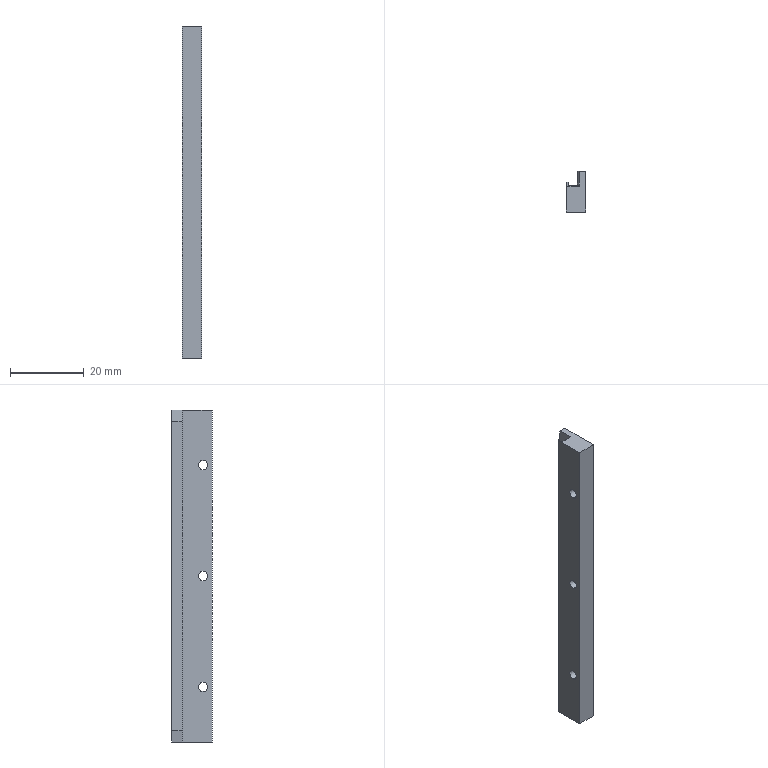Part | NX | features BREP 1 | 1 solid | 22 faces | box 5.3 x 11 x 89.8 mm | volume 4191 mm3 | plane 16 | cylinder 6 | commonest cylinder face diameters 2.5 x6
STEP:
#1=CARTESIAN_POINT('',(3.,11.,41.9));
#2=VERTEX_POINT('',#1);
#3=CARTESIAN_POINT('',(3.5,11.,44.9));
#4=VERTEX_POINT('',#3);
#5=CARTESIAN_POINT('',(3.5,11.,44.9));
#6=DIRECTION('',(0.1644,0.,0.9864));
#7=VECTOR('',#6,1000.);
#8=LINE('',#5,#7);
#9=EDGE_CURVE('',#2,#4,#8,.T.);
#10=ORIENTED_EDGE('',*,*,#9,.F.);
#11=CARTESIAN_POINT('',(3.,7.3,41.9));
#12=VERTEX_POINT('',#11);
#13=CARTESIAN_POINT('',(3.,11.,41.9));
#14=DIRECTION('',(0.,1.,0.));
#15=VECTOR('',#14,1000.);
#16=LINE('',#13,#15);
#17=EDGE_CURVE('',#12,#2,#16,.T.);
#18=ORIENTED_EDGE('',*,*,#17,.F.);
#19=CARTESIAN_POINT('',(3.45,7.3,44.6));
#20=VERTEX_POINT('',#19);
#21=CARTESIAN_POINT('',(3.486,7.3,44.819));
#22=DIRECTION('',(-0.1644,0.,-0.9864));
#23=VECTOR('',#22,1000.);
#24=LINE('',#21,#23);
#25=EDGE_CURVE('',#20,#12,#24,.T.);
#26=ORIENTED_EDGE('',*,*,#25,.F.);
#27=CARTESIAN_POINT('',(3.5,7.,44.9));
#28=VERTEX_POINT('',#27);
#29=CARTESIAN_POINT('',(4.075,3.548,48.352));
#30=DIRECTION('',(-0.117,0.7022,-0.7022));
#31=VECTOR('',#30,1000.);
#32=LINE('',#29,#31);
#33=EDGE_CURVE('',#28,#20,#32,.T.);
#34=ORIENTED_EDGE('',*,*,#33,.F.);
#35=CARTESIAN_POINT('',(3.5,7.,44.9));
#36=DIRECTION('',(0.,-1.,0.));
#37=VECTOR('',#36,1000.);
#38=LINE('',#35,#37);
#39=EDGE_CURVE('',#4,#28,#38,.T.);
#40=ORIENTED_EDGE('',*,*,#39,.F.);
#41=EDGE_LOOP('',(#10,#18,#26,#34,#40));
#42=FACE_BOUND('',#41,.T.);
#43=CARTESIAN_POINT('',(3.5,0.,44.9));
#44=DIRECTION('',(-0.9864,0.,0.1644));
#45=DIRECTION('',(0.,1.,0.));
#46=AXIS2_PLACEMENT_3D('',#43,#44,#45);
#47=PLANE('',#46);
#48=ADVANCED_FACE('',(#42),#47,.T.);
#49=CARTESIAN_POINT('',(3.5,11.,-44.9));
#50=VERTEX_POINT('',#49);
#51=CARTESIAN_POINT('',(3.,11.,-41.9));
#52=VERTEX_POINT('',#51);
#53=CARTESIAN_POINT('',(3.,11.,-41.9));
#54=DIRECTION('',(-0.1644,0.,0.9864));
#55=VECTOR('',#54,1000.);
#56=LINE('',#53,#55);
#57=EDGE_CURVE('',#50,#52,#56,.T.);
#58=ORIENTED_EDGE('',*,*,#57,.F.);
#59=CARTESIAN_POINT('',(3.5,7.,-44.9));
#60=VERTEX_POINT('',#59);
#61=CARTESIAN_POINT('',(3.5,0.,-44.9));
#62=DIRECTION('',(0.,1.,0.));
#63=VECTOR('',#62,1000.);
#64=LINE('',#61,#63);
#65=EDGE_CURVE('',#60,#50,#64,.T.);
#66=ORIENTED_EDGE('',*,*,#65,.F.);
#67=CARTESIAN_POINT('',(3.45,7.3,-44.6));
#68=VERTEX_POINT('',#67);
#69=CARTESIAN_POINT('',(2.918,10.493,-41.407));
#70=DIRECTION('',(0.117,-0.7022,-0.7022));
#71=VECTOR('',#70,1000.);
#72=LINE('',#69,#71);
#73=EDGE_CURVE('',#68,#60,#72,.T.);
#74=ORIENTED_EDGE('',*,*,#73,.F.);
#75=CARTESIAN_POINT('',(3.,7.3,-41.9));
#76=VERTEX_POINT('',#75);
#77=CARTESIAN_POINT('',(-11.076,7.3,42.554));
#78=DIRECTION('',(0.1644,0.,-0.9864));
#79=VECTOR('',#78,1000.);
#80=LINE('',#77,#79);
#81=EDGE_CURVE('',#76,#68,#80,.T.);
#82=ORIENTED_EDGE('',*,*,#81,.F.);
#83=CARTESIAN_POINT('',(3.,11.,-41.9));
#84=DIRECTION('',(0.,-1.,0.));
#85=VECTOR('',#84,1000.);
#86=LINE('',#83,#85);
#87=EDGE_CURVE('',#52,#76,#86,.T.);
#88=ORIENTED_EDGE('',*,*,#87,.F.);
#89=EDGE_LOOP('',(#58,#66,#74,#82,#88));
#90=FACE_BOUND('',#89,.T.);
#91=CARTESIAN_POINT('',(3.,11.,-41.9));
#92=DIRECTION('',(0.9864,0.,0.1644));
#93=DIRECTION('',(0.,-1.,0.));
#94=AXIS2_PLACEMENT_3D('',#91,#92,#93);
#95=PLANE('',#94);
#96=ADVANCED_FACE('',(#90),#95,.F.);
#97=CARTESIAN_POINT('',(0.5,7.3,-44.6));
#98=VERTEX_POINT('',#97);
#99=CARTESIAN_POINT('',(0.2,7.,-44.9));
#100=VERTEX_POINT('',#99);
#101=CARTESIAN_POINT('',(0.5,7.3,-44.6));
#102=DIRECTION('',(-0.5774,-0.5774,-0.5774));
#103=VECTOR('',#102,1000.);
#104=LINE('',#101,#103);
#105=EDGE_CURVE('',#98,#100,#104,.T.);
#106=ORIENTED_EDGE('',*,*,#105,.T.);
#107=CARTESIAN_POINT('',(0.2,8.1,-44.9));
#108=VERTEX_POINT('',#107);
#109=CARTESIAN_POINT('',(0.2,0.,-44.9));
#110=DIRECTION('',(0.,-1.,0.));
#111=VECTOR('',#110,1000.);
#112=LINE('',#109,#111);
#113=EDGE_CURVE('',#108,#100,#112,.T.);
#114=ORIENTED_EDGE('',*,*,#113,.F.);
#115=CARTESIAN_POINT('',(0.5,8.1,-44.6));
#116=VERTEX_POINT('',#115);
#117=CARTESIAN_POINT('',(0.5,8.1,-44.6));
#118=DIRECTION('',(-0.7071,0.,-0.7071));
#119=VECTOR('',#118,1000.);
#120=LINE('',#117,#119);
#121=EDGE_CURVE('',#116,#108,#120,.T.);
#122=ORIENTED_EDGE('',*,*,#121,.F.);
#123=CARTESIAN_POINT('',(0.5,7.3,-44.6));
#124=DIRECTION('',(0.,1.,0.));
#125=VECTOR('',#124,1000.);
#126=LINE('',#123,#125);
#127=EDGE_CURVE('',#98,#116,#126,.T.);
#128=ORIENTED_EDGE('',*,*,#127,.F.);
#129=EDGE_LOOP('',(#106,#114,#122,#128));
#130=FACE_BOUND('',#129,.T.);
#131=CARTESIAN_POINT('',(0.5,7.3,-44.6));
#132=DIRECTION('',(-0.7071,0.,0.7071));
#133=DIRECTION('',(0.,1.,0.));
#134=AXIS2_PLACEMENT_3D('',#131,#132,#133);
#135=PLANE('',#134);
#136=ADVANCED_FACE('',(#130),#135,.F.);
#137=CARTESIAN_POINT('',(3.,7.3,-44.6));
#138=DIRECTION('',(-1.,0.,0.));
#139=VECTOR('',#138,1000.);
#140=LINE('',#137,#139);
#141=EDGE_CURVE('',#68,#98,#140,.T.);
#142=ORIENTED_EDGE('',*,*,#141,.F.);
#143=ORIENTED_EDGE('',*,*,#73,.T.);
#144=CARTESIAN_POINT('',(0.,7.,-44.9));
#145=DIRECTION('',(1.,0.,0.));
#146=VECTOR('',#145,1000.);
#147=LINE('',#144,#146);
#148=EDGE_CURVE('',#100,#60,#147,.T.);
#149=ORIENTED_EDGE('',*,*,#148,.F.);
#150=ORIENTED_EDGE('',*,*,#105,.F.);
#151=EDGE_LOOP('',(#142,#143,#149,#150));
#152=FACE_BOUND('',#151,.T.);
#153=CARTESIAN_POINT('',(3.,7.3,-44.6));
#154=DIRECTION('',(0.,-0.7071,0.7071));
#155=DIRECTION('',(-1.,0.,0.));
#156=AXIS2_PLACEMENT_3D('',#153,#154,#155);
#157=PLANE('',#156);
#158=ADVANCED_FACE('',(#152),#157,.F.);
#159=CARTESIAN_POINT('',(0.2,7.,44.9));
#160=VERTEX_POINT('',#159);
#161=CARTESIAN_POINT('',(0.5,7.3,44.6));
#162=VERTEX_POINT('',#161);
#163=CARTESIAN_POINT('',(-2.133,4.667,47.233));
#164=DIRECTION('',(0.5774,0.5774,-0.5774));
#165=VECTOR('',#164,1000.);
#166=LINE('',#163,#165);
#167=EDGE_CURVE('',#160,#162,#166,.T.);
#168=ORIENTED_EDGE('',*,*,#167,.T.);
#169=CARTESIAN_POINT('',(0.5,8.1,44.6));
#170=VERTEX_POINT('',#169);
#171=CARTESIAN_POINT('',(0.5,7.3,44.6));
#172=DIRECTION('',(0.,-1.,0.));
#173=VECTOR('',#172,1000.);
#174=LINE('',#171,#173);
#175=EDGE_CURVE('',#170,#162,#174,.T.);
#176=ORIENTED_EDGE('',*,*,#175,.F.);
#177=CARTESIAN_POINT('',(0.2,8.1,44.9));
#178=VERTEX_POINT('',#177);
#179=CARTESIAN_POINT('',(0.2,8.1,44.9));
#180=DIRECTION('',(0.7071,0.,-0.7071));
#181=VECTOR('',#180,1000.);
#182=LINE('',#179,#181);
#183=EDGE_CURVE('',#178,#170,#182,.T.);
#184=ORIENTED_EDGE('',*,*,#183,.F.);
#185=CARTESIAN_POINT('',(0.2,8.1,44.9));
#186=DIRECTION('',(0.,1.,0.));
#187=VECTOR('',#186,1000.);
#188=LINE('',#185,#187);
#189=EDGE_CURVE('',#160,#178,#188,.T.);
#190=ORIENTED_EDGE('',*,*,#189,.F.);
#191=EDGE_LOOP('',(#168,#176,#184,#190));
#192=FACE_BOUND('',#191,.T.);
#193=CARTESIAN_POINT('',(0.2,0.,44.9));
#194=DIRECTION('',(0.7071,0.,0.7071));
#195=DIRECTION('',(0.,-1.,0.));
#196=AXIS2_PLACEMENT_3D('',#193,#194,#195);
#197=PLANE('',#196);
#198=ADVANCED_FACE('',(#192),#197,.T.);
#199=CARTESIAN_POINT('',(0.5,7.,44.9));
#200=DIRECTION('',(-1.,0.,0.));
#201=VECTOR('',#200,1000.);
#202=LINE('',#199,#201);
#203=EDGE_CURVE('',#28,#160,#202,.T.);
#204=ORIENTED_EDGE('',*,*,#203,.F.);
#205=ORIENTED_EDGE('',*,*,#33,.T.);
#206=CARTESIAN_POINT('',(3.,7.3,44.6));
#207=DIRECTION('',(1.,0.,0.));
#208=VECTOR('',#207,1000.);
#209=LINE('',#206,#208);
#210=EDGE_CURVE('',#162,#20,#209,.T.);
#211=ORIENTED_EDGE('',*,*,#210,.F.);
#212=ORIENTED_EDGE('',*,*,#167,.F.);
#213=EDGE_LOOP('',(#204,#205,#211,#212));
#214=FACE_BOUND('',#213,.T.);
#215=CARTESIAN_POINT('',(0.,7.,44.9));
#216=DIRECTION('',(0.,0.7071,0.7071));
#217=DIRECTION('',(1.,0.,0.));
#218=AXIS2_PLACEMENT_3D('',#215,#216,#217);
#219=PLANE('',#218);
#220=ADVANCED_FACE('',(#214),#219,.T.);
#221=CARTESIAN_POINT('',(0.,2.5,31.25));
#222=VERTEX_POINT('',#221);
#223=CARTESIAN_POINT('',(5.3,2.5,31.25));
#224=VERTEX_POINT('',#223);
#225=CARTESIAN_POINT('',(5.3,2.5,31.25));
#226=DIRECTION('',(1.,0.,0.));
#227=VECTOR('',#226,1000.);
#228=LINE('',#225,#227);
#229=EDGE_CURVE('',#222,#224,#228,.T.);
#230=ORIENTED_EDGE('',*,*,#229,.F.);
#231=CARTESIAN_POINT('',(0.,2.5,28.75));
#232=VERTEX_POINT('',#231);
#233=CARTESIAN_POINT('',(0.,2.5,30.));
#234=DIRECTION('',(1.,0.,0.));
#235=DIRECTION('',(0.,0.,-1.));
#236=AXIS2_PLACEMENT_3D('',#233,#234,#235);
#237=CIRCLE('',#236,1.25);
#238=EDGE_CURVE('',#232,#222,#237,.T.);
#239=ORIENTED_EDGE('',*,*,#238,.F.);
#240=CARTESIAN_POINT('',(5.3,2.5,28.75));
#241=VERTEX_POINT('',#240);
#242=CARTESIAN_POINT('',(5.3,2.5,28.75));
#243=DIRECTION('',(1.,0.,0.));
#244=VECTOR('',#243,1000.);
#245=LINE('',#242,#244);
#246=EDGE_CURVE('',#232,#241,#245,.T.);
#247=ORIENTED_EDGE('',*,*,#246,.T.);
#248=CARTESIAN_POINT('',(5.3,2.5,30.));
#249=DIRECTION('',(1.,0.,0.));
#250=DIRECTION('',(0.,0.,-1.));
#251=AXIS2_PLACEMENT_3D('',#248,#249,#250);
#252=CIRCLE('',#251,1.25);
#253=EDGE_CURVE('',#241,#224,#252,.T.);
#254=ORIENTED_EDGE('',*,*,#253,.T.);
#255=EDGE_LOOP('',(#230,#239,#247,#254));
#256=FACE_BOUND('',#255,.T.);
#257=CARTESIAN_POINT('',(5.3,2.5,30.));
#258=DIRECTION('',(1.,0.,0.));
#259=DIRECTION('',(0.,0.,-1.));
#260=AXIS2_PLACEMENT_3D('',#257,#258,#259);
#261=CYLINDRICAL_SURFACE('',#260,1.25);
#262=ADVANCED_FACE('',(#256),#261,.F.);
#263=CARTESIAN_POINT('',(0.,2.5,1.25));
#264=VERTEX_POINT('',#263);
#265=CARTESIAN_POINT('',(5.3,2.5,1.25));
#266=VERTEX_POINT('',#265);
#267=CARTESIAN_POINT('',(5.3,2.5,1.25));
#268=DIRECTION('',(1.,0.,0.));
#269=VECTOR('',#268,1000.);
#270=LINE('',#267,#269);
#271=EDGE_CURVE('',#264,#266,#270,.T.);
#272=ORIENTED_EDGE('',*,*,#271,.F.);
#273=CARTESIAN_POINT('',(0.,2.5,-1.25));
#274=VERTEX_POINT('',#273);
#275=CARTESIAN_POINT('',(0.,2.5,0.));
#276=DIRECTION('',(1.,0.,0.));
#277=DIRECTION('',(0.,0.,-1.));
#278=AXIS2_PLACEMENT_3D('',#275,#276,#277);
#279=CIRCLE('',#278,1.25);
#280=EDGE_CURVE('',#274,#264,#279,.T.);
#281=ORIENTED_EDGE('',*,*,#280,.F.);
#282=CARTESIAN_POINT('',(5.3,2.5,-1.25));
#283=VERTEX_POINT('',#282);
#284=CARTESIAN_POINT('',(5.3,2.5,-1.25));
#285=DIRECTION('',(1.,0.,0.));
#286=VECTOR('',#285,1000.);
#287=LINE('',#284,#286);
#288=EDGE_CURVE('',#274,#283,#287,.T.);
#289=ORIENTED_EDGE('',*,*,#288,.T.);
#290=CARTESIAN_POINT('',(5.3,2.5,0.));
#291=DIRECTION('',(1.,0.,0.));
#292=DIRECTION('',(0.,0.,-1.));
#293=AXIS2_PLACEMENT_3D('',#290,#291,#292);
#294=CIRCLE('',#293,1.25);
#295=EDGE_CURVE('',#283,#266,#294,.T.);
#296=ORIENTED_EDGE('',*,*,#295,.T.);
#297=EDGE_LOOP('',(#272,#281,#289,#296));
#298=FACE_BOUND('',#297,.T.);
#299=CARTESIAN_POINT('',(5.3,2.5,0.));
#300=DIRECTION('',(1.,0.,0.));
#301=DIRECTION('',(0.,0.,-1.));
#302=AXIS2_PLACEMENT_3D('',#299,#300,#301);
#303=CYLINDRICAL_SURFACE('',#302,1.25);
#304=ADVANCED_FACE('',(#298),#303,.F.);
#305=CARTESIAN_POINT('',(0.,2.5,-28.75));
#306=VERTEX_POINT('',#305);
#307=CARTESIAN_POINT('',(5.3,2.5,-28.75));
#308=VERTEX_POINT('',#307);
#309=CARTESIAN_POINT('',(5.3,2.5,-28.75));
#310=DIRECTION('',(1.,0.,0.));
#311=VECTOR('',#310,1000.);
#312=LINE('',#309,#311);
#313=EDGE_CURVE('',#306,#308,#312,.T.);
#314=ORIENTED_EDGE('',*,*,#313,.F.);
#315=CARTESIAN_POINT('',(0.,2.5,-31.25));
#316=VERTEX_POINT('',#315);
#317=CARTESIAN_POINT('',(0.,2.5,-30.));
#318=DIRECTION('',(1.,0.,0.));
#319=DIRECTION('',(0.,0.,-1.));
#320=AXIS2_PLACEMENT_3D('',#317,#318,#319);
#321=CIRCLE('',#320,1.25);
#322=EDGE_CURVE('',#316,#306,#321,.T.);
#323=ORIENTED_EDGE('',*,*,#322,.F.);
#324=CARTESIAN_POINT('',(5.3,2.5,-31.25));
#325=VERTEX_POINT('',#324);
#326=CARTESIAN_POINT('',(5.3,2.5,-31.25));
#327=DIRECTION('',(1.,0.,0.));
#328=VECTOR('',#327,1000.);
#329=LINE('',#326,#328);
#330=EDGE_CURVE('',#316,#325,#329,.T.);
#331=ORIENTED_EDGE('',*,*,#330,.T.);
#332=CARTESIAN_POINT('',(5.3,2.5,-30.));
#333=DIRECTION('',(1.,0.,0.));
#334=DIRECTION('',(0.,0.,-1.));
#335=AXIS2_PLACEMENT_3D('',#332,#333,#334);
#336=CIRCLE('',#335,1.25);
#337=EDGE_CURVE('',#325,#308,#336,.T.);
#338=ORIENTED_EDGE('',*,*,#337,.T.);
#339=EDGE_LOOP('',(#314,#323,#331,#338));
#340=FACE_BOUND('',#339,.T.);
#341=CARTESIAN_POINT('',(5.3,2.5,-30.));
#342=DIRECTION('',(1.,0.,0.));
#343=DIRECTION('',(0.,0.,-1.));
#344=AXIS2_PLACEMENT_3D('',#341,#342,#343);
#345=CYLINDRICAL_SURFACE('',#344,1.25);
#346=ADVANCED_FACE('',(#340),#345,.F.);
#347=ORIENTED_EDGE('',*,*,#148,.T.);
#348=ORIENTED_EDGE('',*,*,#65,.T.);
#349=CARTESIAN_POINT('',(5.3,11.,-44.9));
#350=VERTEX_POINT('',#349);
#351=CARTESIAN_POINT('',(5.3,11.,-44.9));
#352=DIRECTION('',(-1.,0.,0.));
#353=VECTOR('',#352,1000.);
#354=LINE('',#351,#353);
#355=EDGE_CURVE('',#350,#50,#354,.T.);
#356=ORIENTED_EDGE('',*,*,#355,.F.);
#357=CARTESIAN_POINT('',(5.3,0.,-44.9));
#358=VERTEX_POINT('',#357);
#359=CARTESIAN_POINT('',(5.3,0.,-44.9));
#360=DIRECTION('',(0.,1.,0.));
#361=VECTOR('',#360,1000.);
#362=LINE('',#359,#361);
#363=EDGE_CURVE('',#358,#350,#362,.T.);
#364=ORIENTED_EDGE('',*,*,#363,.F.);
#365=CARTESIAN_POINT('',(0.,0.,-44.9));
#366=VERTEX_POINT('',#365);
#367=CARTESIAN_POINT('',(0.,0.,-44.9));
#368=DIRECTION('',(1.,0.,0.));
#369=VECTOR('',#368,1000.);
#370=LINE('',#367,#369);
#371=EDGE_CURVE('',#366,#358,#370,.T.);
#372=ORIENTED_EDGE('',*,*,#371,.F.);
#373=CARTESIAN_POINT('',(0.,8.1,-44.9));
#374=VERTEX_POINT('',#373);
#375=CARTESIAN_POINT('',(0.,8.1,-44.9));
#376=DIRECTION('',(0.,-1.,0.));
#377=VECTOR('',#376,1000.);
#378=LINE('',#375,#377);
#379=EDGE_CURVE('',#374,#366,#378,.T.);
#380=ORIENTED_EDGE('',*,*,#379,.F.);
#381=CARTESIAN_POINT('',(0.5,8.1,-44.9));
#382=DIRECTION('',(-1.,0.,0.));
#383=VECTOR('',#382,1000.);
#384=LINE('',#381,#383);
#385=EDGE_CURVE('',#108,#374,#384,.T.);
#386=ORIENTED_EDGE('',*,*,#385,.F.);
#387=ORIENTED_EDGE('',*,*,#113,.T.);
#388=EDGE_LOOP('',(#347,#348,#356,#364,#372,#380,#386,#387));
#389=FACE_BOUND('',#388,.T.);
#390=CARTESIAN_POINT('',(0.,0.,-44.9));
#391=DIRECTION('',(0.,0.,1.));
#392=DIRECTION('',(1.,0.,0.));
#393=AXIS2_PLACEMENT_3D('',#390,#391,#392);
#394=PLANE('',#393);
#395=ADVANCED_FACE('',(#389),#394,.F.);
#396=CARTESIAN_POINT('',(5.3,11.,44.9));
#397=VERTEX_POINT('',#396);
#398=CARTESIAN_POINT('',(5.3,11.,44.9));
#399=DIRECTION('',(-1.,0.,0.));
#400=VECTOR('',#399,1000.);
#401=LINE('',#398,#400);
#402=EDGE_CURVE('',#397,#4,#401,.T.);
#403=ORIENTED_EDGE('',*,*,#402,.T.);
#404=ORIENTED_EDGE('',*,*,#39,.T.);
#405=ORIENTED_EDGE('',*,*,#203,.T.);
#406=ORIENTED_EDGE('',*,*,#189,.T.);
#407=CARTESIAN_POINT('',(0.,8.1,44.9));
#408=VERTEX_POINT('',#407);
#409=CARTESIAN_POINT('',(0.5,8.1,44.9));
#410=DIRECTION('',(-1.,0.,0.));
#411=VECTOR('',#410,1000.);
#412=LINE('',#409,#411);
#413=EDGE_CURVE('',#178,#408,#412,.T.);
#414=ORIENTED_EDGE('',*,*,#413,.T.);
#415=CARTESIAN_POINT('',(0.,0.,44.9));
#416=VERTEX_POINT('',#415);
#417=CARTESIAN_POINT('',(0.,8.1,44.9));
#418=DIRECTION('',(0.,-1.,0.));
#419=VECTOR('',#418,1000.);
#420=LINE('',#417,#419);
#421=EDGE_CURVE('',#408,#416,#420,.T.);
#422=ORIENTED_EDGE('',*,*,#421,.T.);
#423=CARTESIAN_POINT('',(5.3,0.,44.9));
#424=VERTEX_POINT('',#423);
#425=CARTESIAN_POINT('',(0.,0.,44.9));
#426=DIRECTION('',(1.,0.,0.));
#427=VECTOR('',#426,1000.);
#428=LINE('',#425,#427);
#429=EDGE_CURVE('',#416,#424,#428,.T.);
#430=ORIENTED_EDGE('',*,*,#429,.T.);
#431=CARTESIAN_POINT('',(5.3,0.,44.9));
#432=DIRECTION('',(0.,1.,0.));
#433=VECTOR('',#432,1000.);
#434=LINE('',#431,#433);
#435=EDGE_CURVE('',#424,#397,#434,.T.);
#436=ORIENTED_EDGE('',*,*,#435,.T.);
#437=EDGE_LOOP('',(#403,#404,#405,#406,#414,#422,#430,#436));
#438=FACE_BOUND('',#437,.T.);
#439=CARTESIAN_POINT('',(0.,0.,44.9));
#440=DIRECTION('',(0.,0.,1.));
#441=DIRECTION('',(1.,0.,0.));
#442=AXIS2_PLACEMENT_3D('',#439,#440,#441);
#443=PLANE('',#442);
#444=ADVANCED_FACE('',(#438),#443,.T.);
#445=ORIENTED_EDGE('',*,*,#413,.F.);
#446=ORIENTED_EDGE('',*,*,#183,.T.);
#447=CARTESIAN_POINT('',(0.5,8.1,44.9));
#448=DIRECTION('',(0.,0.,-1.));
#449=VECTOR('',#448,1000.);
#450=LINE('',#447,#449);
#451=EDGE_CURVE('',#170,#116,#450,.T.);
#452=ORIENTED_EDGE('',*,*,#451,.T.);
#453=ORIENTED_EDGE('',*,*,#121,.T.);
#454=ORIENTED_EDGE('',*,*,#385,.T.);
#455=CARTESIAN_POINT('',(0.,8.1,44.9));
#456=DIRECTION('',(0.,0.,-1.));
#457=VECTOR('',#456,1000.);
#458=LINE('',#455,#457);
#459=EDGE_CURVE('',#408,#374,#458,.T.);
#460=ORIENTED_EDGE('',*,*,#459,.F.);
#461=EDGE_LOOP('',(#445,#446,#452,#453,#454,#460));
#462=FACE_BOUND('',#461,.T.);
#463=CARTESIAN_POINT('',(0.5,8.1,44.9));
#464=DIRECTION('',(0.,-1.,0.));
#465=DIRECTION('',(0.,0.,-1.));
#466=AXIS2_PLACEMENT_3D('',#463,#464,#465);
#467=PLANE('',#466);
#468=ADVANCED_FACE('',(#462),#467,.F.);
#469=ORIENTED_EDGE('',*,*,#451,.F.);
#470=ORIENTED_EDGE('',*,*,#175,.T.);
#471=CARTESIAN_POINT('',(0.5,7.3,44.9));
#472=DIRECTION('',(0.,0.,-1.));
#473=VECTOR('',#472,1000.);
#474=LINE('',#471,#473);
#475=EDGE_CURVE('',#162,#98,#474,.T.);
#476=ORIENTED_EDGE('',*,*,#475,.T.);
#477=ORIENTED_EDGE('',*,*,#127,.T.);
#478=EDGE_LOOP('',(#469,#470,#476,#477));
#479=FACE_BOUND('',#478,.T.);
#480=CARTESIAN_POINT('',(0.5,7.3,44.9));
#481=DIRECTION('',(-1.,0.,0.));
#482=DIRECTION('',(0.,-1.,0.));
#483=AXIS2_PLACEMENT_3D('',#480,#481,#482);
#484=PLANE('',#483);
#485=ADVANCED_FACE('',(#479),#484,.F.);
#486=ORIENTED_EDGE('',*,*,#475,.F.);
#487=ORIENTED_EDGE('',*,*,#210,.T.);
#488=ORIENTED_EDGE('',*,*,#25,.T.);
#489=CARTESIAN_POINT('',(3.,7.3,44.9));
#490=DIRECTION('',(0.,0.,-1.));
#491=VECTOR('',#490,1000.);
#492=LINE('',#489,#491);
#493=EDGE_CURVE('',#12,#76,#492,.T.);
#494=ORIENTED_EDGE('',*,*,#493,.T.);
#495=ORIENTED_EDGE('',*,*,#81,.T.);
#496=ORIENTED_EDGE('',*,*,#141,.T.);
#497=EDGE_LOOP('',(#486,#487,#488,#494,#495,#496));
#498=FACE_BOUND('',#497,.T.);
#499=CARTESIAN_POINT('',(3.,7.3,44.9));
#500=DIRECTION('',(0.,-1.,0.));
#501=DIRECTION('',(1.,0.,0.));
#502=AXIS2_PLACEMENT_3D('',#499,#500,#501);
#503=PLANE('',#502);
#504=ADVANCED_FACE('',(#498),#503,.F.);
#505=CARTESIAN_POINT('',(3.,11.,44.9));
#506=DIRECTION('',(0.,0.,-1.));
#507=VECTOR('',#506,1000.);
#508=LINE('',#505,#507);
#509=EDGE_CURVE('',#2,#52,#508,.T.);
#510=ORIENTED_EDGE('',*,*,#509,.T.);
#511=ORIENTED_EDGE('',*,*,#87,.T.);
#512=ORIENTED_EDGE('',*,*,#493,.F.);
#513=ORIENTED_EDGE('',*,*,#17,.T.);
#514=EDGE_LOOP('',(#510,#511,#512,#513));
#515=FACE_BOUND('',#514,.T.);
#516=CARTESIAN_POINT('',(3.,11.,44.9));
#517=DIRECTION('',(1.,0.,0.));
#518=DIRECTION('',(0.,1.,0.));
#519=AXIS2_PLACEMENT_3D('',#516,#517,#518);
#520=PLANE('',#519);
#521=ADVANCED_FACE('',(#515),#520,.F.);
#522=ORIENTED_EDGE('',*,*,#355,.T.);
#523=ORIENTED_EDGE('',*,*,#57,.T.);
#524=ORIENTED_EDGE('',*,*,#509,.F.);
#525=ORIENTED_EDGE('',*,*,#9,.T.);
#526=ORIENTED_EDGE('',*,*,#402,.F.);
#527=CARTESIAN_POINT('',(5.3,11.,44.9));
#528=DIRECTION('',(0.,0.,-1.));
#529=VECTOR('',#528,1000.);
#530=LINE('',#527,#529);
#531=EDGE_CURVE('',#397,#350,#530,.T.);
#532=ORIENTED_EDGE('',*,*,#531,.T.);
#533=EDGE_LOOP('',(#522,#523,#524,#525,#526,#532));
#534=FACE_BOUND('',#533,.T.);
#535=CARTESIAN_POINT('',(5.3,11.,44.9));
#536=DIRECTION('',(0.,-1.,0.));
#537=DIRECTION('',(0.,0.,-1.));
#538=AXIS2_PLACEMENT_3D('',#535,#536,#537);
#539=PLANE('',#538);
#540=ADVANCED_FACE('',(#534),#539,.F.);
#541=ORIENTED_EDGE('',*,*,#363,.T.);
#542=ORIENTED_EDGE('',*,*,#531,.F.);
#543=ORIENTED_EDGE('',*,*,#435,.F.);
#544=CARTESIAN_POINT('',(5.3,0.,44.9));
#545=DIRECTION('',(0.,0.,-1.));
#546=VECTOR('',#545,1000.);
#547=LINE('',#544,#546);
#548=EDGE_CURVE('',#424,#358,#547,.T.);
#549=ORIENTED_EDGE('',*,*,#548,.T.);
#550=EDGE_LOOP('',(#541,#542,#543,#549));
#551=FACE_BOUND('',#550,.T.);
#552=ORIENTED_EDGE('',*,*,#337,.F.);
#553=CARTESIAN_POINT('',(5.3,2.5,-30.));
#554=DIRECTION('',(1.,0.,0.));
#555=DIRECTION('',(0.,0.,-1.));
#556=AXIS2_PLACEMENT_3D('',#553,#554,#555);
#557=CIRCLE('',#556,1.25);
#558=EDGE_CURVE('',#308,#325,#557,.T.);
#559=ORIENTED_EDGE('',*,*,#558,.F.);
#560=EDGE_LOOP('',(#552,#559));
#561=FACE_BOUND('',#560,.T.);
#562=ORIENTED_EDGE('',*,*,#295,.F.);
#563=CARTESIAN_POINT('',(5.3,2.5,0.));
#564=DIRECTION('',(1.,0.,0.));
#565=DIRECTION('',(0.,0.,-1.));
#566=AXIS2_PLACEMENT_3D('',#563,#564,#565);
#567=CIRCLE('',#566,1.25);
#568=EDGE_CURVE('',#266,#283,#567,.T.);
#569=ORIENTED_EDGE('',*,*,#568,.F.);
#570=EDGE_LOOP('',(#562,#569));
#571=FACE_BOUND('',#570,.T.);
#572=ORIENTED_EDGE('',*,*,#253,.F.);
#573=CARTESIAN_POINT('',(5.3,2.5,30.));
#574=DIRECTION('',(1.,0.,0.));
#575=DIRECTION('',(0.,0.,-1.));
#576=AXIS2_PLACEMENT_3D('',#573,#574,#575);
#577=CIRCLE('',#576,1.25);
#578=EDGE_CURVE('',#224,#241,#577,.T.);
#579=ORIENTED_EDGE('',*,*,#578,.F.);
#580=EDGE_LOOP('',(#572,#579));
#581=FACE_BOUND('',#580,.T.);
#582=CARTESIAN_POINT('',(5.3,0.,44.9));
#583=DIRECTION('',(-1.,0.,0.));
#584=DIRECTION('',(0.,-1.,0.));
#585=AXIS2_PLACEMENT_3D('',#582,#583,#584);
#586=PLANE('',#585);
#587=ADVANCED_FACE('',(#551,#561,#571,#581),#586,.F.);
#588=ORIENTED_EDGE('',*,*,#371,.T.);
#589=ORIENTED_EDGE('',*,*,#548,.F.);
#590=ORIENTED_EDGE('',*,*,#429,.F.);
#591=CARTESIAN_POINT('',(0.,0.,44.9));
#592=DIRECTION('',(0.,0.,-1.));
#593=VECTOR('',#592,1000.);
#594=LINE('',#591,#593);
#595=EDGE_CURVE('',#416,#366,#594,.T.);
#596=ORIENTED_EDGE('',*,*,#595,.T.);
#597=EDGE_LOOP('',(#588,#589,#590,#596));
#598=FACE_BOUND('',#597,.T.);
#599=CARTESIAN_POINT('',(0.,0.,44.9));
#600=DIRECTION('',(0.,1.,0.));
#601=DIRECTION('',(0.,0.,1.));
#602=AXIS2_PLACEMENT_3D('',#599,#600,#601);
#603=PLANE('',#602);
#604=ADVANCED_FACE('',(#598),#603,.F.);
#605=ORIENTED_EDGE('',*,*,#379,.T.);
#606=ORIENTED_EDGE('',*,*,#595,.F.);
#607=ORIENTED_EDGE('',*,*,#421,.F.);
#608=ORIENTED_EDGE('',*,*,#459,.T.);
#609=EDGE_LOOP('',(#605,#606,#607,#608));
#610=FACE_BOUND('',#609,.T.);
#611=ORIENTED_EDGE('',*,*,#322,.T.);
#612=CARTESIAN_POINT('',(0.,2.5,-30.));
#613=DIRECTION('',(1.,0.,0.));
#614=DIRECTION('',(0.,0.,-1.));
#615=AXIS2_PLACEMENT_3D('',#612,#613,#614);
#616=CIRCLE('',#615,1.25);
#617=EDGE_CURVE('',#306,#316,#616,.T.);
#618=ORIENTED_EDGE('',*,*,#617,.T.);
#619=EDGE_LOOP('',(#611,#618));
#620=FACE_BOUND('',#619,.T.);
#621=ORIENTED_EDGE('',*,*,#280,.T.);
#622=CARTESIAN_POINT('',(0.,2.5,0.));
#623=DIRECTION('',(1.,0.,0.));
#624=DIRECTION('',(0.,0.,-1.));
#625=AXIS2_PLACEMENT_3D('',#622,#623,#624);
#626=CIRCLE('',#625,1.25);
#627=EDGE_CURVE('',#264,#274,#626,.T.);
#628=ORIENTED_EDGE('',*,*,#627,.T.);
#629=EDGE_LOOP('',(#621,#628));
#630=FACE_BOUND('',#629,.T.);
#631=ORIENTED_EDGE('',*,*,#238,.T.);
#632=CARTESIAN_POINT('',(0.,2.5,30.));
#633=DIRECTION('',(1.,0.,0.));
#634=DIRECTION('',(0.,0.,-1.));
#635=AXIS2_PLACEMENT_3D('',#632,#633,#634);
#636=CIRCLE('',#635,1.25);
#637=EDGE_CURVE('',#222,#232,#636,.T.);
#638=ORIENTED_EDGE('',*,*,#637,.T.);
#639=EDGE_LOOP('',(#631,#638));
#640=FACE_BOUND('',#639,.T.);
#641=CARTESIAN_POINT('',(0.,8.1,44.9));
#642=DIRECTION('',(1.,0.,0.));
#643=DIRECTION('',(0.,1.,0.));
#644=AXIS2_PLACEMENT_3D('',#641,#642,#643);
#645=PLANE('',#644);
#646=ADVANCED_FACE('',(#610,#620,#630,#640),#645,.F.);
#647=ORIENTED_EDGE('',*,*,#617,.F.);
#648=ORIENTED_EDGE('',*,*,#313,.T.);
#649=ORIENTED_EDGE('',*,*,#558,.T.);
#650=ORIENTED_EDGE('',*,*,#330,.F.);
#651=EDGE_LOOP('',(#647,#648,#649,#650));
#652=FACE_BOUND('',#651,.T.);
#653=CARTESIAN_POINT('',(5.3,2.5,-30.));
#654=DIRECTION('',(1.,0.,0.));
#655=DIRECTION('',(0.,0.,-1.));
#656=AXIS2_PLACEMENT_3D('',#653,#654,#655);
#657=CYLINDRICAL_SURFACE('',#656,1.25);
#658=ADVANCED_FACE('',(#652),#657,.F.);
#659=ORIENTED_EDGE('',*,*,#627,.F.);
#660=ORIENTED_EDGE('',*,*,#271,.T.);
#661=ORIENTED_EDGE('',*,*,#568,.T.);
#662=ORIENTED_EDGE('',*,*,#288,.F.);
#663=EDGE_LOOP('',(#659,#660,#661,#662));
#664=FACE_BOUND('',#663,.T.);
#665=CARTESIAN_POINT('',(5.3,2.5,0.));
#666=DIRECTION('',(1.,0.,0.));
#667=DIRECTION('',(0.,0.,-1.));
#668=AXIS2_PLACEMENT_3D('',#665,#666,#667);
#669=CYLINDRICAL_SURFACE('',#668,1.25);
#670=ADVANCED_FACE('',(#664),#669,.F.);
#671=ORIENTED_EDGE('',*,*,#637,.F.);
#672=ORIENTED_EDGE('',*,*,#229,.T.);
#673=ORIENTED_EDGE('',*,*,#578,.T.);
#674=ORIENTED_EDGE('',*,*,#246,.F.);
#675=EDGE_LOOP('',(#671,#672,#673,#674));
#676=FACE_BOUND('',#675,.T.);
#677=CARTESIAN_POINT('',(5.3,2.5,30.));
#678=DIRECTION('',(1.,0.,0.));
#679=DIRECTION('',(0.,0.,-1.));
#680=AXIS2_PLACEMENT_3D('',#677,#678,#679);
#681=CYLINDRICAL_SURFACE('',#680,1.25);
#682=ADVANCED_FACE('',(#676),#681,.F.);
#683=CLOSED_SHELL('',(#48,#96,#136,#158,#198,#220,#262,#304,#346,#395,#444,#468,#485,#504,#521,#540,#587,#604,#646,#658,#670,#682));
#684=MANIFOLD_SOLID_BREP('',#683);
#685=(LENGTH_UNIT()NAMED_UNIT(*)SI_UNIT(.MILLI.,.METRE.));
#686=UNCERTAINTY_MEASURE_WITH_UNIT(LENGTH_MEASURE(0.00001),#685,'','');
#687=(NAMED_UNIT(*)PLANE_ANGLE_UNIT()SI_UNIT($,.RADIAN.));
#688=(NAMED_UNIT(*)SI_UNIT($,.STERADIAN.)SOLID_ANGLE_UNIT());
#689=(GEOMETRIC_REPRESENTATION_CONTEXT(3)GLOBAL_UNCERTAINTY_ASSIGNED_CONTEXT((#686))GLOBAL_UNIT_ASSIGNED_CONTEXT((#685,#687,#688))REPRESENTATION_CONTEXT('',''));
#690=ADVANCED_BREP_SHAPE_REPRESENTATION('',(#684),#689);